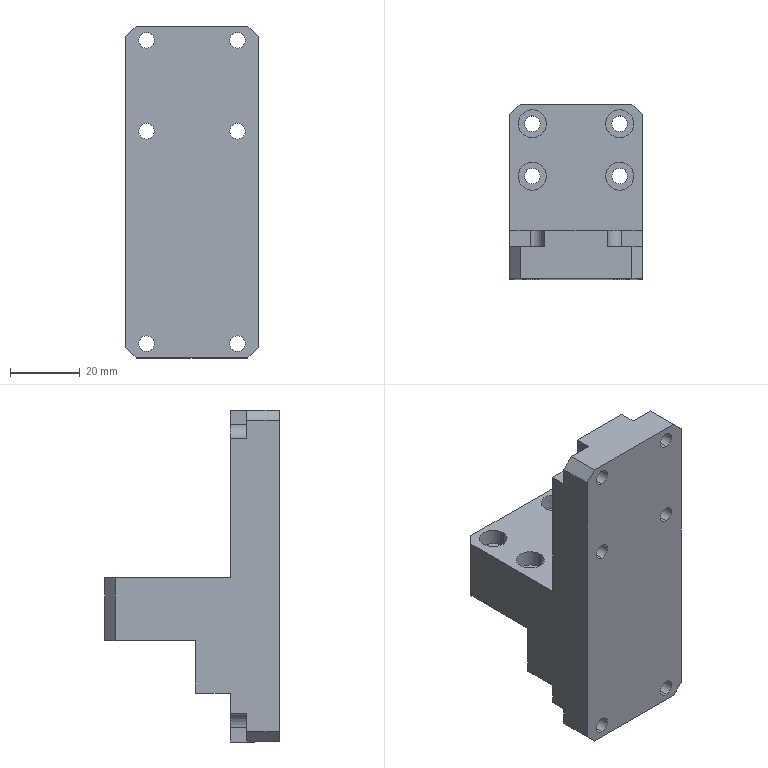Part | STEP file | FBDS-CS-013 | 1 solid | 72 faces | box 38 x 50 x 95 mm | volume 75969 mm3 | cylinder 36 | plane 36 | commonest cylinder face diameters 4.5 x20 8 x16